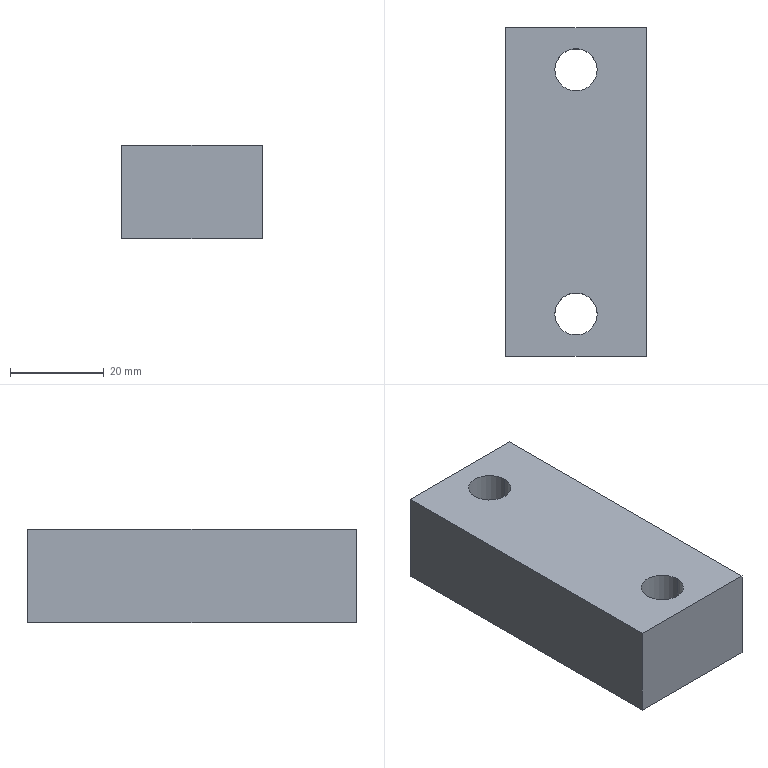Part | STEP file | X77-04013 | 1 solid | 10 faces | box 30 x 70 x 20 mm | volume 39455 mm3 | plane 6 | cylinder 4 | commonest cylinder face diameters 9 x4
STEP:
#1=CARTESIAN_POINT('',(-322.5,17.349,0.));
#2=VERTEX_POINT('',#1);
#3=CARTESIAN_POINT('',(-313.5,17.349,0.));
#4=VERTEX_POINT('',#3);
#5=CARTESIAN_POINT('',(-318.,17.349,0.));
#6=DIRECTION('',(0.,0.,1.));
#7=DIRECTION('',(1.,0.,0.));
#8=AXIS2_PLACEMENT_3D('',#5,#6,#7);
#9=CIRCLE('',#8,4.5);
#10=EDGE_CURVE('',#2,#4,#9,.T.);
#11=ORIENTED_EDGE('',*,*,#10,.F.);
#12=CARTESIAN_POINT('',(-322.5,17.349,20.));
#13=VERTEX_POINT('',#12);
#14=CARTESIAN_POINT('',(-322.5,17.349,0.));
#15=DIRECTION('',(0.,0.,1.));
#16=VECTOR('',#15,1000.);
#17=LINE('',#14,#16);
#18=EDGE_CURVE('',#2,#13,#17,.T.);
#19=ORIENTED_EDGE('',*,*,#18,.T.);
#20=CARTESIAN_POINT('',(-313.5,17.349,20.));
#21=VERTEX_POINT('',#20);
#22=CARTESIAN_POINT('',(-318.,17.349,20.));
#23=DIRECTION('',(0.,0.,1.));
#24=DIRECTION('',(1.,0.,0.));
#25=AXIS2_PLACEMENT_3D('',#22,#23,#24);
#26=CIRCLE('',#25,4.5);
#27=EDGE_CURVE('',#13,#21,#26,.T.);
#28=ORIENTED_EDGE('',*,*,#27,.T.);
#29=CARTESIAN_POINT('',(-313.5,17.349,0.));
#30=DIRECTION('',(0.,0.,1.));
#31=VECTOR('',#30,1000.);
#32=LINE('',#29,#31);
#33=EDGE_CURVE('',#4,#21,#32,.T.);
#34=ORIENTED_EDGE('',*,*,#33,.F.);
#35=EDGE_LOOP('',(#11,#19,#28,#34));
#36=FACE_OUTER_BOUND('',#35,.T.);
#37=CARTESIAN_POINT('',(-318.,17.349,0.));
#38=DIRECTION('',(0.,0.,1.));
#39=DIRECTION('',(1.,0.,0.));
#40=AXIS2_PLACEMENT_3D('',#37,#38,#39);
#41=CYLINDRICAL_SURFACE('',#40,4.5);
#42=ADVANCED_FACE('',(#36),#41,.F.);
#43=CARTESIAN_POINT('',(-322.5,69.349,0.));
#44=VERTEX_POINT('',#43);
#45=CARTESIAN_POINT('',(-313.5,69.349,0.));
#46=VERTEX_POINT('',#45);
#47=CARTESIAN_POINT('',(-318.,69.349,0.));
#48=DIRECTION('',(0.,0.,1.));
#49=DIRECTION('',(1.,0.,0.));
#50=AXIS2_PLACEMENT_3D('',#47,#48,#49);
#51=CIRCLE('',#50,4.5);
#52=EDGE_CURVE('',#44,#46,#51,.T.);
#53=ORIENTED_EDGE('',*,*,#52,.F.);
#54=CARTESIAN_POINT('',(-322.5,69.349,20.));
#55=VERTEX_POINT('',#54);
#56=CARTESIAN_POINT('',(-322.5,69.349,0.));
#57=DIRECTION('',(0.,0.,1.));
#58=VECTOR('',#57,1000.);
#59=LINE('',#56,#58);
#60=EDGE_CURVE('',#44,#55,#59,.T.);
#61=ORIENTED_EDGE('',*,*,#60,.T.);
#62=CARTESIAN_POINT('',(-313.5,69.349,20.));
#63=VERTEX_POINT('',#62);
#64=CARTESIAN_POINT('',(-318.,69.349,20.));
#65=DIRECTION('',(0.,0.,1.));
#66=DIRECTION('',(1.,0.,0.));
#67=AXIS2_PLACEMENT_3D('',#64,#65,#66);
#68=CIRCLE('',#67,4.5);
#69=EDGE_CURVE('',#55,#63,#68,.T.);
#70=ORIENTED_EDGE('',*,*,#69,.T.);
#71=CARTESIAN_POINT('',(-313.5,69.349,0.));
#72=DIRECTION('',(0.,0.,1.));
#73=VECTOR('',#72,1000.);
#74=LINE('',#71,#73);
#75=EDGE_CURVE('',#46,#63,#74,.T.);
#76=ORIENTED_EDGE('',*,*,#75,.F.);
#77=EDGE_LOOP('',(#53,#61,#70,#76));
#78=FACE_OUTER_BOUND('',#77,.T.);
#79=CARTESIAN_POINT('',(-318.,69.349,0.));
#80=DIRECTION('',(0.,0.,1.));
#81=DIRECTION('',(1.,0.,0.));
#82=AXIS2_PLACEMENT_3D('',#79,#80,#81);
#83=CYLINDRICAL_SURFACE('',#82,4.5);
#84=ADVANCED_FACE('',(#78),#83,.F.);
#85=CARTESIAN_POINT('',(-303.,78.349,0.));
#86=VERTEX_POINT('',#85);
#87=CARTESIAN_POINT('',(-333.,78.349,0.));
#88=VERTEX_POINT('',#87);
#89=CARTESIAN_POINT('',(-333.,78.349,0.));
#90=DIRECTION('',(-1.,0.,0.));
#91=VECTOR('',#90,1000.);
#92=LINE('',#89,#91);
#93=EDGE_CURVE('',#86,#88,#92,.T.);
#94=ORIENTED_EDGE('',*,*,#93,.T.);
#95=CARTESIAN_POINT('',(-333.,78.349,20.));
#96=VERTEX_POINT('',#95);
#97=CARTESIAN_POINT('',(-333.,78.349,20.));
#98=DIRECTION('',(0.,0.,-1.));
#99=VECTOR('',#98,1000.);
#100=LINE('',#97,#99);
#101=EDGE_CURVE('',#96,#88,#100,.T.);
#102=ORIENTED_EDGE('',*,*,#101,.F.);
#103=CARTESIAN_POINT('',(-303.,78.349,20.));
#104=VERTEX_POINT('',#103);
#105=CARTESIAN_POINT('',(-333.,78.349,20.));
#106=DIRECTION('',(-1.,0.,0.));
#107=VECTOR('',#106,1000.);
#108=LINE('',#105,#107);
#109=EDGE_CURVE('',#104,#96,#108,.T.);
#110=ORIENTED_EDGE('',*,*,#109,.F.);
#111=CARTESIAN_POINT('',(-303.,78.349,20.));
#112=DIRECTION('',(0.,0.,-1.));
#113=VECTOR('',#112,1000.);
#114=LINE('',#111,#113);
#115=EDGE_CURVE('',#104,#86,#114,.T.);
#116=ORIENTED_EDGE('',*,*,#115,.T.);
#117=EDGE_LOOP('',(#94,#102,#110,#116));
#118=FACE_OUTER_BOUND('',#117,.T.);
#119=CARTESIAN_POINT('',(-333.,78.349,20.));
#120=DIRECTION('',(0.,-1.,0.));
#121=DIRECTION('',(0.,0.,-1.));
#122=AXIS2_PLACEMENT_3D('',#119,#120,#121);
#123=PLANE('',#122);
#124=ADVANCED_FACE('',(#118),#123,.F.);
#125=CARTESIAN_POINT('',(-333.,8.349,0.));
#126=VERTEX_POINT('',#125);
#127=CARTESIAN_POINT('',(-333.,78.349,0.));
#128=DIRECTION('',(0.,-1.,0.));
#129=VECTOR('',#128,1000.);
#130=LINE('',#127,#129);
#131=EDGE_CURVE('',#88,#126,#130,.T.);
#132=ORIENTED_EDGE('',*,*,#131,.T.);
#133=CARTESIAN_POINT('',(-333.,8.349,20.));
#134=VERTEX_POINT('',#133);
#135=CARTESIAN_POINT('',(-333.,8.349,20.));
#136=DIRECTION('',(0.,0.,-1.));
#137=VECTOR('',#136,1000.);
#138=LINE('',#135,#137);
#139=EDGE_CURVE('',#134,#126,#138,.T.);
#140=ORIENTED_EDGE('',*,*,#139,.F.);
#141=CARTESIAN_POINT('',(-333.,78.349,20.));
#142=DIRECTION('',(0.,-1.,0.));
#143=VECTOR('',#142,1000.);
#144=LINE('',#141,#143);
#145=EDGE_CURVE('',#96,#134,#144,.T.);
#146=ORIENTED_EDGE('',*,*,#145,.F.);
#147=ORIENTED_EDGE('',*,*,#101,.T.);
#148=EDGE_LOOP('',(#132,#140,#146,#147));
#149=FACE_OUTER_BOUND('',#148,.T.);
#150=CARTESIAN_POINT('',(-333.,78.349,20.));
#151=DIRECTION('',(1.,0.,0.));
#152=DIRECTION('',(0.,0.,-1.));
#153=AXIS2_PLACEMENT_3D('',#150,#151,#152);
#154=PLANE('',#153);
#155=ADVANCED_FACE('',(#149),#154,.F.);
#156=CARTESIAN_POINT('',(-303.,8.349,0.));
#157=VERTEX_POINT('',#156);
#158=CARTESIAN_POINT('',(-333.,8.349,0.));
#159=DIRECTION('',(1.,0.,0.));
#160=VECTOR('',#159,1000.);
#161=LINE('',#158,#160);
#162=EDGE_CURVE('',#126,#157,#161,.T.);
#163=ORIENTED_EDGE('',*,*,#162,.T.);
#164=CARTESIAN_POINT('',(-303.,8.349,20.));
#165=VERTEX_POINT('',#164);
#166=CARTESIAN_POINT('',(-303.,8.349,20.));
#167=DIRECTION('',(0.,0.,-1.));
#168=VECTOR('',#167,1000.);
#169=LINE('',#166,#168);
#170=EDGE_CURVE('',#165,#157,#169,.T.);
#171=ORIENTED_EDGE('',*,*,#170,.F.);
#172=CARTESIAN_POINT('',(-333.,8.349,20.));
#173=DIRECTION('',(1.,0.,0.));
#174=VECTOR('',#173,1000.);
#175=LINE('',#172,#174);
#176=EDGE_CURVE('',#134,#165,#175,.T.);
#177=ORIENTED_EDGE('',*,*,#176,.F.);
#178=ORIENTED_EDGE('',*,*,#139,.T.);
#179=EDGE_LOOP('',(#163,#171,#177,#178));
#180=FACE_OUTER_BOUND('',#179,.T.);
#181=CARTESIAN_POINT('',(-333.,8.349,20.));
#182=DIRECTION('',(0.,1.,0.));
#183=DIRECTION('',(-1.,0.,0.));
#184=AXIS2_PLACEMENT_3D('',#181,#182,#183);
#185=PLANE('',#184);
#186=ADVANCED_FACE('',(#180),#185,.F.);
#187=CARTESIAN_POINT('',(-303.,78.349,0.));
#188=DIRECTION('',(0.,1.,0.));
#189=VECTOR('',#188,1000.);
#190=LINE('',#187,#189);
#191=EDGE_CURVE('',#157,#86,#190,.T.);
#192=ORIENTED_EDGE('',*,*,#191,.T.);
#193=ORIENTED_EDGE('',*,*,#115,.F.);
#194=CARTESIAN_POINT('',(-303.,78.349,20.));
#195=DIRECTION('',(0.,1.,0.));
#196=VECTOR('',#195,1000.);
#197=LINE('',#194,#196);
#198=EDGE_CURVE('',#165,#104,#197,.T.);
#199=ORIENTED_EDGE('',*,*,#198,.F.);
#200=ORIENTED_EDGE('',*,*,#170,.T.);
#201=EDGE_LOOP('',(#192,#193,#199,#200));
#202=FACE_OUTER_BOUND('',#201,.T.);
#203=CARTESIAN_POINT('',(-303.,78.349,20.));
#204=DIRECTION('',(-1.,0.,0.));
#205=DIRECTION('',(0.,0.,1.));
#206=AXIS2_PLACEMENT_3D('',#203,#204,#205);
#207=PLANE('',#206);
#208=ADVANCED_FACE('',(#202),#207,.F.);
#209=CARTESIAN_POINT('',(-318.,17.349,20.));
#210=DIRECTION('',(0.,0.,1.));
#211=DIRECTION('',(1.,0.,0.));
#212=AXIS2_PLACEMENT_3D('',#209,#210,#211);
#213=CIRCLE('',#212,4.5);
#214=EDGE_CURVE('',#21,#13,#213,.T.);
#215=ORIENTED_EDGE('',*,*,#214,.F.);
#216=ORIENTED_EDGE('',*,*,#27,.F.);
#217=EDGE_LOOP('',(#215,#216));
#218=FACE_BOUND('',#217,.T.);
#219=CARTESIAN_POINT('',(-318.,69.349,20.));
#220=DIRECTION('',(0.,0.,1.));
#221=DIRECTION('',(1.,0.,0.));
#222=AXIS2_PLACEMENT_3D('',#219,#220,#221);
#223=CIRCLE('',#222,4.5);
#224=EDGE_CURVE('',#63,#55,#223,.T.);
#225=ORIENTED_EDGE('',*,*,#224,.F.);
#226=ORIENTED_EDGE('',*,*,#69,.F.);
#227=EDGE_LOOP('',(#225,#226));
#228=FACE_BOUND('',#227,.T.);
#229=ORIENTED_EDGE('',*,*,#109,.T.);
#230=ORIENTED_EDGE('',*,*,#145,.T.);
#231=ORIENTED_EDGE('',*,*,#176,.T.);
#232=ORIENTED_EDGE('',*,*,#198,.T.);
#233=EDGE_LOOP('',(#229,#230,#231,#232));
#234=FACE_OUTER_BOUND('',#233,.T.);
#235=CARTESIAN_POINT('',(-303.,78.349,20.));
#236=DIRECTION('',(0.,0.,-1.));
#237=DIRECTION('',(-1.,0.,0.));
#238=AXIS2_PLACEMENT_3D('',#235,#236,#237);
#239=PLANE('',#238);
#240=ADVANCED_FACE('',(#218,#228,#234),#239,.F.);
#241=CARTESIAN_POINT('',(-318.,17.349,0.));
#242=DIRECTION('',(0.,0.,1.));
#243=DIRECTION('',(1.,0.,0.));
#244=AXIS2_PLACEMENT_3D('',#241,#242,#243);
#245=CIRCLE('',#244,4.5);
#246=EDGE_CURVE('',#4,#2,#245,.T.);
#247=ORIENTED_EDGE('',*,*,#246,.T.);
#248=ORIENTED_EDGE('',*,*,#10,.T.);
#249=EDGE_LOOP('',(#247,#248));
#250=FACE_BOUND('',#249,.T.);
#251=CARTESIAN_POINT('',(-318.,69.349,0.));
#252=DIRECTION('',(0.,0.,1.));
#253=DIRECTION('',(1.,0.,0.));
#254=AXIS2_PLACEMENT_3D('',#251,#252,#253);
#255=CIRCLE('',#254,4.5);
#256=EDGE_CURVE('',#46,#44,#255,.T.);
#257=ORIENTED_EDGE('',*,*,#256,.T.);
#258=ORIENTED_EDGE('',*,*,#52,.T.);
#259=EDGE_LOOP('',(#257,#258));
#260=FACE_BOUND('',#259,.T.);
#261=ORIENTED_EDGE('',*,*,#93,.F.);
#262=ORIENTED_EDGE('',*,*,#191,.F.);
#263=ORIENTED_EDGE('',*,*,#162,.F.);
#264=ORIENTED_EDGE('',*,*,#131,.F.);
#265=EDGE_LOOP('',(#261,#262,#263,#264));
#266=FACE_OUTER_BOUND('',#265,.T.);
#267=CARTESIAN_POINT('',(-303.,78.349,0.));
#268=DIRECTION('',(0.,0.,-1.));
#269=DIRECTION('',(-1.,0.,0.));
#270=AXIS2_PLACEMENT_3D('',#267,#268,#269);
#271=PLANE('',#270);
#272=ADVANCED_FACE('',(#250,#260,#266),#271,.T.);
#273=ORIENTED_EDGE('',*,*,#60,.F.);
#274=ORIENTED_EDGE('',*,*,#256,.F.);
#275=ORIENTED_EDGE('',*,*,#75,.T.);
#276=ORIENTED_EDGE('',*,*,#224,.T.);
#277=EDGE_LOOP('',(#273,#274,#275,#276));
#278=FACE_OUTER_BOUND('',#277,.T.);
#279=CARTESIAN_POINT('',(-318.,69.349,0.));
#280=DIRECTION('',(0.,0.,1.));
#281=DIRECTION('',(1.,0.,0.));
#282=AXIS2_PLACEMENT_3D('',#279,#280,#281);
#283=CYLINDRICAL_SURFACE('',#282,4.5);
#284=ADVANCED_FACE('',(#278),#283,.F.);
#285=ORIENTED_EDGE('',*,*,#18,.F.);
#286=ORIENTED_EDGE('',*,*,#246,.F.);
#287=ORIENTED_EDGE('',*,*,#33,.T.);
#288=ORIENTED_EDGE('',*,*,#214,.T.);
#289=EDGE_LOOP('',(#285,#286,#287,#288));
#290=FACE_OUTER_BOUND('',#289,.T.);
#291=CARTESIAN_POINT('',(-318.,17.349,0.));
#292=DIRECTION('',(0.,0.,1.));
#293=DIRECTION('',(1.,0.,0.));
#294=AXIS2_PLACEMENT_3D('',#291,#292,#293);
#295=CYLINDRICAL_SURFACE('',#294,4.5);
#296=ADVANCED_FACE('',(#290),#295,.F.);
#297=CLOSED_SHELL('',(#42,#84,#124,#155,#186,#208,#240,#272,#284,#296));
#298=MANIFOLD_SOLID_BREP('',#297);
#299=CARTESIAN_POINT('',(0.,0.,0.));
#300=DIRECTION('',(0.,0.,1.));
#301=DIRECTION('',(1.,0.,0.));
#302=AXIS2_PLACEMENT_3D('',#299,#300,#301);
#303=(LENGTH_UNIT()NAMED_UNIT(*)SI_UNIT(.MILLI.,.METRE.));
#304=UNCERTAINTY_MEASURE_WITH_UNIT(LENGTH_MEASURE(0.00001),#303,'','');
#305=(NAMED_UNIT(*)PLANE_ANGLE_UNIT()SI_UNIT($,.RADIAN.));
#306=(NAMED_UNIT(*)SI_UNIT($,.STERADIAN.)SOLID_ANGLE_UNIT());
#307=(GEOMETRIC_REPRESENTATION_CONTEXT(3)GLOBAL_UNCERTAINTY_ASSIGNED_CONTEXT((#304))GLOBAL_UNIT_ASSIGNED_CONTEXT((#303,#305,#306))REPRESENTATION_CONTEXT('',''));
#308=ADVANCED_BREP_SHAPE_REPRESENTATION('',(#298,#302),#307);